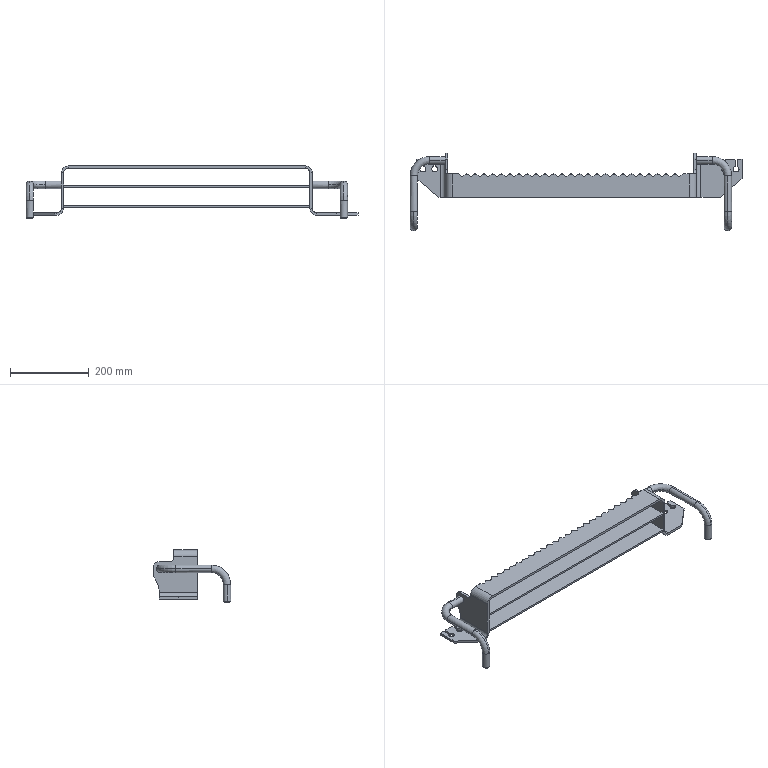Part | SolidWorks | features BaseBody 5 | 5 solids | 240 faces | box 841.5 x 196.5 x 132.5 mm | volume 877492 mm3 | plane 121 | cylinder 107 | torus 8 | cone 4 | commonest cylinder face diameters 4 x53 15 x12 19 x12 2 x8 6 x8 24 x4